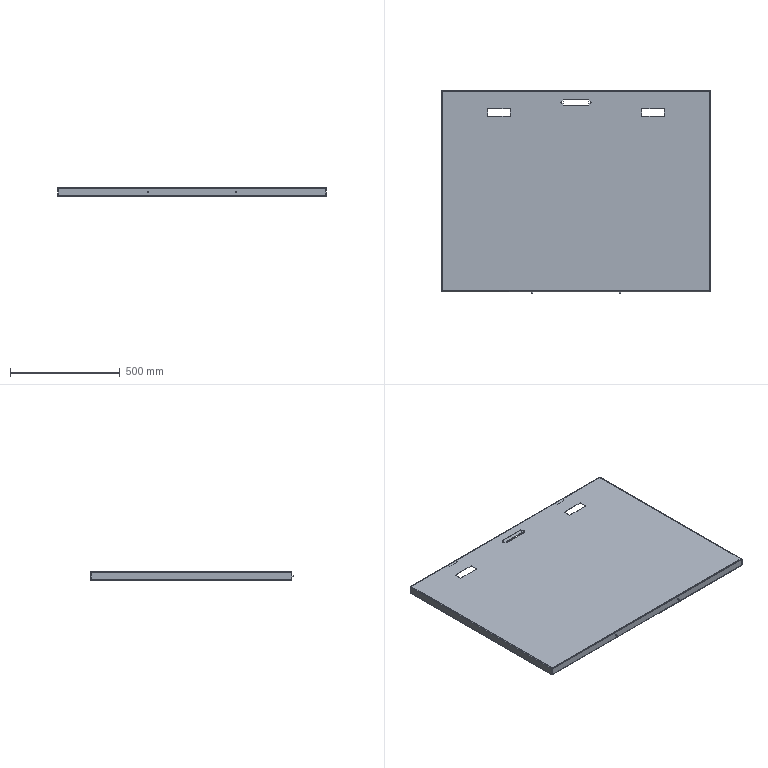Part | SolidWorks | features ICE 6, SMWeldBead 4, EdgeFlange 2, FlatPattern 1, HoleWzd 1, SMBaseFlange 1, SheetMetal 1 | 3 solids | 177 faces | box 1225 x 925 x 38 mm | volume 2035721 mm3 | plane 102 | spline 40 | cylinder 35 | commonest cylinder face diameters 4 x12 7 x10 6 x6 2 x4 9 x3